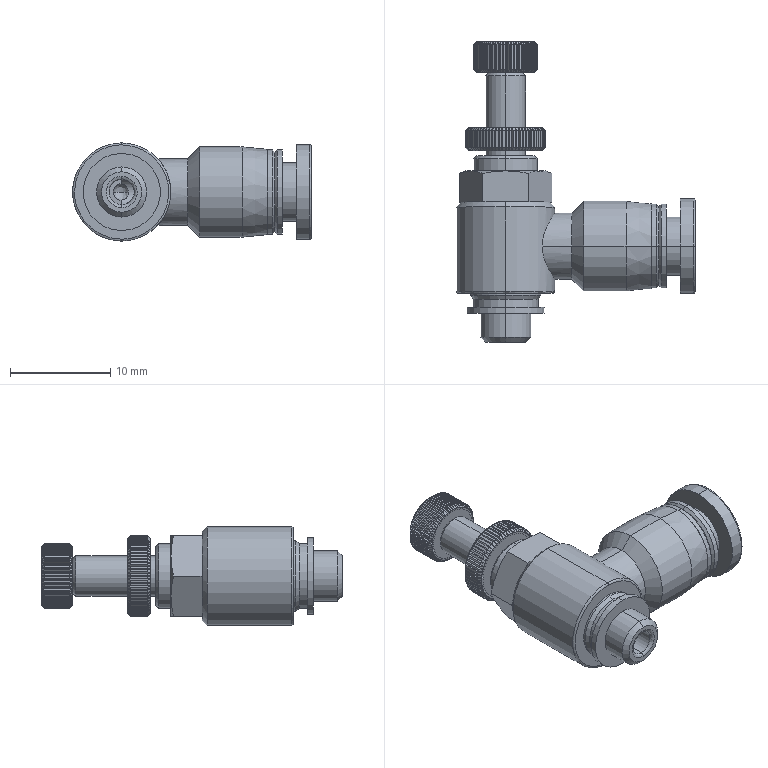Part | STEP file | Tube-fitting one-way flow control valve AirTAC ASL4-M5-1 | 1 solid | 839 faces | box 23.8 x 30 x 9.8 mm | volume 1827 mm3 | plane 336 | cone 312 | cylinder 181 | spline 10 | commonest cylinder face diameters 6.4 x74 8 x72 4 x6 8.4 x4 2.5 x2 2.667 x2